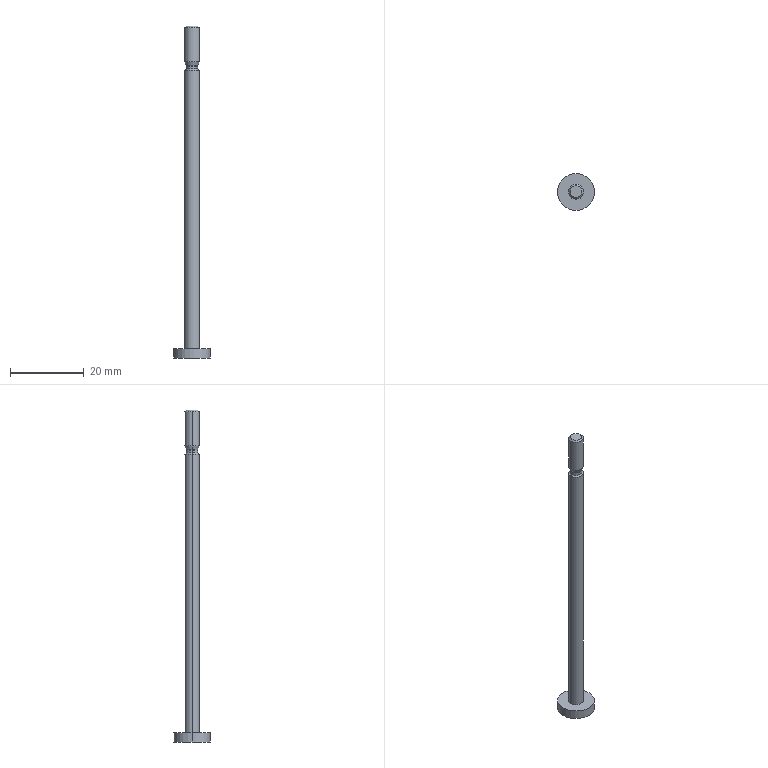Part | STEP file | PN_0050 | 1 solid | 19 faces | box 10 x 10 x 90 mm | volume 1287 mm3 | cylinder 8 | cone 4 | torus 4 | plane 3 | commonest cylinder face diameters 4 x4 3.2 x2 10 x2
STEP:
#1=CARTESIAN_POINT('',(0.,0.,0.));
#2=DIRECTION('',(0.,0.,1.));
#3=DIRECTION('',(1.,0.,0.));
#4=AXIS2_PLACEMENT_3D('',#1,#2,#3);
#5=CARTESIAN_POINT('',(1.571,0.,16.));
#6=VERTEX_POINT('',#5);
#7=CARTESIAN_POINT('',(-1.571,0.,16.));
#8=VERTEX_POINT('',#7);
#9=CARTESIAN_POINT('',(0.,0.,16.));
#10=DIRECTION('',(0.,0.,1.));
#11=DIRECTION('',(1.,0.,0.));
#12=AXIS2_PLACEMENT_3D('',#9,#10,#11);
#13=CIRCLE('',#12,1.571);
#14=CARTESIAN_POINT('',(0.,0.,15.57));
#15=DIRECTION('',(0.,0.,-1.));
#16=DIRECTION('',(-1.,0.,0.));
#17=AXIS2_PLACEMENT_3D('',#14,#15,#16);
#18=CONICAL_SURFACE('',#17,2.,0.7854);
#19=CARTESIAN_POINT('',(3.142,-0.4295));
#20=DIRECTION('',(-1.,0.));
#21=VECTOR('',#20,1.);
#22=LINE('',#19,#21);
#23=(GEOMETRIC_REPRESENTATION_CONTEXT(2)PARAMETRIC_REPRESENTATION_CONTEXT()REPRESENTATION_CONTEXT('',''));
#24=DEFINITIONAL_REPRESENTATION('',(#22),#23);
#25=PCURVE('',#18,#24);
#26=CARTESIAN_POINT('',(0.,0.,16.));
#27=DIRECTION('',(0.,0.,-1.));
#28=DIRECTION('',(-1.,0.,0.));
#29=AXIS2_PLACEMENT_3D('',#26,#27,#28);
#30=PLANE('',#29);
#31=CARTESIAN_POINT('',(-1.571,0.));
#32=CARTESIAN_POINT('',(-1.571,2.72));
#33=CARTESIAN_POINT('',(0.7853,1.36));
#34=CARTESIAN_POINT('',(3.141,0.));
#35=CARTESIAN_POINT('',(0.7853,-1.36));
#36=CARTESIAN_POINT('',(-1.571,-2.72));
#37=CARTESIAN_POINT('',(-1.571,0.));
#38=(BOUNDED_CURVE()B_SPLINE_CURVE(2,(#31,#32,#33,#34,#35,#36,#37),.UNSPECIFIED.,.T.,.F.)B_SPLINE_CURVE_WITH_KNOTS((1,2,2,2,2,1),(-2.094,0.,2.094,4.189,6.283,8.378),.UNSPECIFIED.)CURVE()GEOMETRIC_REPRESENTATION_ITEM()RATIONAL_B_SPLINE_CURVE((1.,0.5,1.,0.5,1.,0.5,1.))REPRESENTATION_ITEM(''));
#39=(GEOMETRIC_REPRESENTATION_CONTEXT(2)PARAMETRIC_REPRESENTATION_CONTEXT()REPRESENTATION_CONTEXT('',''));
#40=DEFINITIONAL_REPRESENTATION('',(#38),#39);
#41=PCURVE('',#30,#40);
#42=SURFACE_CURVE('',#13,(#25,#41),.PCURVE_S1.);
#43=EDGE_CURVE('',#6,#8,#42,.T.);
#44=ORIENTED_EDGE('',*,*,#43,.F.);
#45=CARTESIAN_POINT('',(2.,0.,15.57));
#46=VERTEX_POINT('',#45);
#47=CARTESIAN_POINT('',(2.,0.,15.57));
#48=DIRECTION('',(0.7071,0.,-0.7071));
#49=VECTOR('',#48,1.);
#50=LINE('',#47,#49);
#51=CARTESIAN_POINT('',(3.142,0.));
#52=DIRECTION('',(0.,1.));
#53=VECTOR('',#52,1.);
#54=LINE('',#51,#53);
#55=(GEOMETRIC_REPRESENTATION_CONTEXT(2)PARAMETRIC_REPRESENTATION_CONTEXT()REPRESENTATION_CONTEXT('',''));
#56=DEFINITIONAL_REPRESENTATION('',(#54),#55);
#57=PCURVE('',#18,#56);
#58=CARTESIAN_POINT('',(0.,0.,15.57));
#59=DIRECTION('',(0.,0.,-1.));
#60=DIRECTION('',(-1.,0.,0.));
#61=AXIS2_PLACEMENT_3D('',#58,#59,#60);
#62=CONICAL_SURFACE('',#61,2.,0.7854);
#63=CARTESIAN_POINT('',(3.142,0.));
#64=DIRECTION('',(0.,1.));
#65=VECTOR('',#64,1.);
#66=LINE('',#63,#65);
#67=(GEOMETRIC_REPRESENTATION_CONTEXT(2)PARAMETRIC_REPRESENTATION_CONTEXT()REPRESENTATION_CONTEXT('',''));
#68=DEFINITIONAL_REPRESENTATION('',(#66),#67);
#69=PCURVE('',#62,#68);
#70=SURFACE_CURVE('',#50,(#57,#69),.PCURVE_S1.);
#71=EDGE_CURVE('',#6,#46,#70,.T.);
#72=ORIENTED_EDGE('',*,*,#71,.T.);
#73=CARTESIAN_POINT('',(-2.,0.,15.57));
#74=VERTEX_POINT('',#73);
#75=CARTESIAN_POINT('',(0.,0.,15.57));
#76=DIRECTION('',(0.,0.,1.));
#77=DIRECTION('',(1.,0.,0.));
#78=AXIS2_PLACEMENT_3D('',#75,#76,#77);
#79=CIRCLE('',#78,2.);
#80=CARTESIAN_POINT('',(3.142,0.));
#81=DIRECTION('',(-1.,0.));
#82=VECTOR('',#81,1.);
#83=LINE('',#80,#82);
#84=(GEOMETRIC_REPRESENTATION_CONTEXT(2)PARAMETRIC_REPRESENTATION_CONTEXT()REPRESENTATION_CONTEXT('',''));
#85=DEFINITIONAL_REPRESENTATION('',(#83),#84);
#86=PCURVE('',#18,#85);
#87=CARTESIAN_POINT('',(0.,0.,3.));
#88=DIRECTION('',(0.,0.,1.));
#89=DIRECTION('',(1.,0.,0.));
#90=AXIS2_PLACEMENT_3D('',#87,#88,#89);
#91=CYLINDRICAL_SURFACE('',#90,2.);
#92=CARTESIAN_POINT('',(0.,12.57));
#93=DIRECTION('',(1.,0.));
#94=VECTOR('',#93,1.);
#95=LINE('',#92,#94);
#96=(GEOMETRIC_REPRESENTATION_CONTEXT(2)PARAMETRIC_REPRESENTATION_CONTEXT()REPRESENTATION_CONTEXT('',''));
#97=DEFINITIONAL_REPRESENTATION('',(#95),#96);
#98=PCURVE('',#91,#97);
#99=SURFACE_CURVE('',#79,(#86,#98),.PCURVE_S1.);
#100=EDGE_CURVE('',#46,#74,#99,.T.);
#101=ORIENTED_EDGE('',*,*,#100,.T.);
#102=CARTESIAN_POINT('',(-2.,0.,15.57));
#103=DIRECTION('',(-0.7071,0.,-0.7071));
#104=VECTOR('',#103,1.);
#105=LINE('',#102,#104);
#106=CARTESIAN_POINT('',(0.,0.));
#107=DIRECTION('',(0.,1.));
#108=VECTOR('',#107,1.);
#109=LINE('',#106,#108);
#110=(GEOMETRIC_REPRESENTATION_CONTEXT(2)PARAMETRIC_REPRESENTATION_CONTEXT()REPRESENTATION_CONTEXT('',''));
#111=DEFINITIONAL_REPRESENTATION('',(#109),#110);
#112=PCURVE('',#18,#111);
#113=CARTESIAN_POINT('',(6.283,0.));
#114=DIRECTION('',(0.,1.));
#115=VECTOR('',#114,1.);
#116=LINE('',#113,#115);
#117=(GEOMETRIC_REPRESENTATION_CONTEXT(2)PARAMETRIC_REPRESENTATION_CONTEXT()REPRESENTATION_CONTEXT('',''));
#118=DEFINITIONAL_REPRESENTATION('',(#116),#117);
#119=PCURVE('',#62,#118);
#120=SURFACE_CURVE('',#105,(#112,#119),.PCURVE_S1.);
#121=EDGE_CURVE('',#8,#74,#120,.T.);
#122=ORIENTED_EDGE('',*,*,#121,.F.);
#123=EDGE_LOOP('',(#44,#72,#101,#122));
#124=FACE_BOUND('',#123,.T.);
#125=ADVANCED_FACE('',(#124),#18,.T.);
#126=CARTESIAN_POINT('',(2.,0.,6.299));
#127=VERTEX_POINT('',#126);
#128=CARTESIAN_POINT('',(-2.,0.,6.299));
#129=VERTEX_POINT('',#128);
#130=CARTESIAN_POINT('',(0.,0.,6.299));
#131=DIRECTION('',(0.,0.,1.));
#132=DIRECTION('',(1.,0.,0.));
#133=AXIS2_PLACEMENT_3D('',#130,#131,#132);
#134=CIRCLE('',#133,2.);
#135=CARTESIAN_POINT('',(0.,3.299));
#136=DIRECTION('',(1.,0.));
#137=VECTOR('',#136,1.);
#138=LINE('',#135,#137);
#139=(GEOMETRIC_REPRESENTATION_CONTEXT(2)PARAMETRIC_REPRESENTATION_CONTEXT()REPRESENTATION_CONTEXT('',''));
#140=DEFINITIONAL_REPRESENTATION('',(#138),#139);
#141=PCURVE('',#91,#140);
#142=CARTESIAN_POINT('',(0.,0.,5.266));
#143=DIRECTION('',(0.,0.,1.));
#144=DIRECTION('',(1.,0.,0.));
#145=AXIS2_PLACEMENT_3D('',#142,#143,#144);
#146=CONICAL_SURFACE('',#145,1.624,0.3491);
#147=CARTESIAN_POINT('',(0.,1.033));
#148=DIRECTION('',(1.,0.));
#149=VECTOR('',#148,1.);
#150=LINE('',#147,#149);
#151=(GEOMETRIC_REPRESENTATION_CONTEXT(2)PARAMETRIC_REPRESENTATION_CONTEXT()REPRESENTATION_CONTEXT('',''));
#152=DEFINITIONAL_REPRESENTATION('',(#150),#151);
#153=PCURVE('',#146,#152);
#154=SURFACE_CURVE('',#134,(#141,#153),.PCURVE_S1.);
#155=EDGE_CURVE('',#127,#129,#154,.T.);
#156=ORIENTED_EDGE('',*,*,#155,.T.);
#157=CARTESIAN_POINT('',(-2.,0.,3.));
#158=DIRECTION('',(0.,0.,1.));
#159=VECTOR('',#158,1.);
#160=LINE('',#157,#159);
#161=CARTESIAN_POINT('',(3.142,0.));
#162=DIRECTION('',(0.,1.));
#163=VECTOR('',#162,1.);
#164=LINE('',#161,#163);
#165=(GEOMETRIC_REPRESENTATION_CONTEXT(2)PARAMETRIC_REPRESENTATION_CONTEXT()REPRESENTATION_CONTEXT('',''));
#166=DEFINITIONAL_REPRESENTATION('',(#164),#165);
#167=PCURVE('',#91,#166);
#168=CARTESIAN_POINT('',(0.,0.,3.));
#169=DIRECTION('',(0.,0.,1.));
#170=DIRECTION('',(1.,0.,0.));
#171=AXIS2_PLACEMENT_3D('',#168,#169,#170);
#172=CYLINDRICAL_SURFACE('',#171,2.);
#173=CARTESIAN_POINT('',(3.142,0.));
#174=DIRECTION('',(0.,1.));
#175=VECTOR('',#174,1.);
#176=LINE('',#173,#175);
#177=(GEOMETRIC_REPRESENTATION_CONTEXT(2)PARAMETRIC_REPRESENTATION_CONTEXT()REPRESENTATION_CONTEXT('',''));
#178=DEFINITIONAL_REPRESENTATION('',(#176),#177);
#179=PCURVE('',#172,#178);
#180=SURFACE_CURVE('',#160,(#167,#179),.PCURVE_S1.);
#181=EDGE_CURVE('',#129,#74,#180,.T.);
#182=ORIENTED_EDGE('',*,*,#181,.T.);
#183=ORIENTED_EDGE('',*,*,#100,.F.);
#184=CARTESIAN_POINT('',(2.,0.,3.));
#185=DIRECTION('',(0.,0.,1.));
#186=VECTOR('',#185,1.);
#187=LINE('',#184,#186);
#188=CARTESIAN_POINT('',(0.,0.));
#189=DIRECTION('',(0.,1.));
#190=VECTOR('',#189,1.);
#191=LINE('',#188,#190);
#192=(GEOMETRIC_REPRESENTATION_CONTEXT(2)PARAMETRIC_REPRESENTATION_CONTEXT()REPRESENTATION_CONTEXT('',''));
#193=DEFINITIONAL_REPRESENTATION('',(#191),#192);
#194=PCURVE('',#91,#193);
#195=CARTESIAN_POINT('',(6.283,0.));
#196=DIRECTION('',(0.,1.));
#197=VECTOR('',#196,1.);
#198=LINE('',#195,#197);
#199=(GEOMETRIC_REPRESENTATION_CONTEXT(2)PARAMETRIC_REPRESENTATION_CONTEXT()REPRESENTATION_CONTEXT('',''));
#200=DEFINITIONAL_REPRESENTATION('',(#198),#199);
#201=PCURVE('',#172,#200);
#202=SURFACE_CURVE('',#187,(#194,#201),.PCURVE_S1.);
#203=EDGE_CURVE('',#127,#46,#202,.T.);
#204=ORIENTED_EDGE('',*,*,#203,.F.);
#205=EDGE_LOOP('',(#156,#182,#183,#204));
#206=FACE_BOUND('',#205,.T.);
#207=ADVANCED_FACE('',(#206),#91,.T.);
#208=CARTESIAN_POINT('',(1.624,0.,5.266));
#209=VERTEX_POINT('',#208);
#210=CARTESIAN_POINT('',(-1.624,0.,5.266));
#211=VERTEX_POINT('',#210);
#212=CARTESIAN_POINT('',(0.,0.,5.266));
#213=DIRECTION('',(0.,0.,1.));
#214=DIRECTION('',(1.,0.,0.));
#215=AXIS2_PLACEMENT_3D('',#212,#213,#214);
#216=CIRCLE('',#215,1.624);
#217=CARTESIAN_POINT('',(0.,0.));
#218=DIRECTION('',(1.,0.));
#219=VECTOR('',#218,1.);
#220=LINE('',#217,#219);
#221=(GEOMETRIC_REPRESENTATION_CONTEXT(2)PARAMETRIC_REPRESENTATION_CONTEXT()REPRESENTATION_CONTEXT('',''));
#222=DEFINITIONAL_REPRESENTATION('',(#220),#221);
#223=PCURVE('',#146,#222);
#224=CARTESIAN_POINT('',(0.,0.,5.129));
#225=DIRECTION('',(0.,0.,1.));
#226=DIRECTION('',(1.,0.,0.));
#227=AXIS2_PLACEMENT_3D('',#224,#225,#226);
#228=TOROIDAL_SURFACE('',#227,2.,0.4);
#229=CARTESIAN_POINT('',(0.,2.793));
#230=DIRECTION('',(1.,0.));
#231=VECTOR('',#230,1.);
#232=LINE('',#229,#231);
#233=(GEOMETRIC_REPRESENTATION_CONTEXT(2)PARAMETRIC_REPRESENTATION_CONTEXT()REPRESENTATION_CONTEXT('',''));
#234=DEFINITIONAL_REPRESENTATION('',(#232),#233);
#235=PCURVE('',#228,#234);
#236=SURFACE_CURVE('',#216,(#223,#235),.PCURVE_S1.);
#237=EDGE_CURVE('',#209,#211,#236,.T.);
#238=ORIENTED_EDGE('',*,*,#237,.T.);
#239=CARTESIAN_POINT('',(-1.624,0.,5.266));
#240=DIRECTION('',(-0.342,0.,0.9397));
#241=VECTOR('',#240,1.);
#242=LINE('',#239,#241);
#243=CARTESIAN_POINT('',(3.142,0.));
#244=DIRECTION('',(0.,1.));
#245=VECTOR('',#244,1.);
#246=LINE('',#243,#245);
#247=(GEOMETRIC_REPRESENTATION_CONTEXT(2)PARAMETRIC_REPRESENTATION_CONTEXT()REPRESENTATION_CONTEXT('',''));
#248=DEFINITIONAL_REPRESENTATION('',(#246),#247);
#249=PCURVE('',#146,#248);
#250=CARTESIAN_POINT('',(0.,0.,5.266));
#251=DIRECTION('',(0.,0.,1.));
#252=DIRECTION('',(1.,0.,0.));
#253=AXIS2_PLACEMENT_3D('',#250,#251,#252);
#254=CONICAL_SURFACE('',#253,1.624,0.3491);
#255=CARTESIAN_POINT('',(3.142,0.));
#256=DIRECTION('',(0.,1.));
#257=VECTOR('',#256,1.);
#258=LINE('',#255,#257);
#259=(GEOMETRIC_REPRESENTATION_CONTEXT(2)PARAMETRIC_REPRESENTATION_CONTEXT()REPRESENTATION_CONTEXT('',''));
#260=DEFINITIONAL_REPRESENTATION('',(#258),#259);
#261=PCURVE('',#254,#260);
#262=SURFACE_CURVE('',#242,(#249,#261),.PCURVE_S1.);
#263=EDGE_CURVE('',#211,#129,#262,.T.);
#264=ORIENTED_EDGE('',*,*,#263,.T.);
#265=ORIENTED_EDGE('',*,*,#155,.F.);
#266=CARTESIAN_POINT('',(1.624,0.,5.266));
#267=DIRECTION('',(0.342,0.,0.9397));
#268=VECTOR('',#267,1.);
#269=LINE('',#266,#268);
#270=CARTESIAN_POINT('',(0.,0.));
#271=DIRECTION('',(0.,1.));
#272=VECTOR('',#271,1.);
#273=LINE('',#270,#272);
#274=(GEOMETRIC_REPRESENTATION_CONTEXT(2)PARAMETRIC_REPRESENTATION_CONTEXT()REPRESENTATION_CONTEXT('',''));
#275=DEFINITIONAL_REPRESENTATION('',(#273),#274);
#276=PCURVE('',#146,#275);
#277=CARTESIAN_POINT('',(6.283,0.));
#278=DIRECTION('',(0.,1.));
#279=VECTOR('',#278,1.);
#280=LINE('',#277,#279);
#281=(GEOMETRIC_REPRESENTATION_CONTEXT(2)PARAMETRIC_REPRESENTATION_CONTEXT()REPRESENTATION_CONTEXT('',''));
#282=DEFINITIONAL_REPRESENTATION('',(#280),#281);
#283=PCURVE('',#254,#282);
#284=SURFACE_CURVE('',#269,(#276,#283),.PCURVE_S1.);
#285=EDGE_CURVE('',#209,#127,#284,.T.);
#286=ORIENTED_EDGE('',*,*,#285,.F.);
#287=EDGE_LOOP('',(#238,#264,#265,#286));
#288=FACE_BOUND('',#287,.T.);
#289=ADVANCED_FACE('',(#288),#146,.T.);
#290=CARTESIAN_POINT('',(1.6,0.,5.129));
#291=VERTEX_POINT('',#290);
#292=CARTESIAN_POINT('',(2.,0.,5.129));
#293=DIRECTION('',(0.,-1.,0.));
#294=DIRECTION('',(0.,0.,-1.));
#295=AXIS2_PLACEMENT_3D('',#292,#293,#294);
#296=CIRCLE('',#295,0.4);
#297=CARTESIAN_POINT('',(0.,0.,5.129));
#298=DIRECTION('',(0.,0.,1.));
#299=DIRECTION('',(1.,0.,0.));
#300=AXIS2_PLACEMENT_3D('',#297,#298,#299);
#301=TOROIDAL_SURFACE('',#300,2.,0.4);
#302=CARTESIAN_POINT('',(6.283,-1.571));
#303=DIRECTION('',(0.,1.));
#304=VECTOR('',#303,1.);
#305=LINE('',#302,#304);
#306=(GEOMETRIC_REPRESENTATION_CONTEXT(2)PARAMETRIC_REPRESENTATION_CONTEXT()REPRESENTATION_CONTEXT('',''));
#307=DEFINITIONAL_REPRESENTATION('',(#305),#306);
#308=PCURVE('',#301,#307);
#309=CARTESIAN_POINT('',(0.,-1.571));
#310=DIRECTION('',(0.,1.));
#311=VECTOR('',#310,1.);
#312=LINE('',#309,#311);
#313=(GEOMETRIC_REPRESENTATION_CONTEXT(2)PARAMETRIC_REPRESENTATION_CONTEXT()REPRESENTATION_CONTEXT('',''));
#314=DEFINITIONAL_REPRESENTATION('',(#312),#313);
#315=PCURVE('',#228,#314);
#316=SURFACE_CURVE('',#296,(#308,#315),.PCURVE_S1.);
#317=EDGE_CURVE('',#209,#291,#316,.T.);
#318=ORIENTED_EDGE('',*,*,#317,.T.);
#319=CARTESIAN_POINT('',(-1.6,0.,5.129));
#320=VERTEX_POINT('',#319);
#321=CARTESIAN_POINT('',(0.,0.,5.129));
#322=DIRECTION('',(0.,0.,1.));
#323=DIRECTION('',(1.,0.,0.));
#324=AXIS2_PLACEMENT_3D('',#321,#322,#323);
#325=CIRCLE('',#324,1.6);
#326=CARTESIAN_POINT('',(0.,3.142));
#327=DIRECTION('',(1.,0.));
#328=VECTOR('',#327,1.);
#329=LINE('',#326,#328);
#330=(GEOMETRIC_REPRESENTATION_CONTEXT(2)PARAMETRIC_REPRESENTATION_CONTEXT()REPRESENTATION_CONTEXT('',''));
#331=DEFINITIONAL_REPRESENTATION('',(#329),#330);
#332=PCURVE('',#301,#331);
#333=CARTESIAN_POINT('',(0.,0.,3.));
#334=DIRECTION('',(0.,0.,1.));
#335=DIRECTION('',(1.,0.,0.));
#336=AXIS2_PLACEMENT_3D('',#333,#334,#335);
#337=CYLINDRICAL_SURFACE('',#336,1.6);
#338=CARTESIAN_POINT('',(0.,2.129));
#339=DIRECTION('',(1.,0.));
#340=VECTOR('',#339,1.);
#341=LINE('',#338,#340);
#342=(GEOMETRIC_REPRESENTATION_CONTEXT(2)PARAMETRIC_REPRESENTATION_CONTEXT()REPRESENTATION_CONTEXT('',''));
#343=DEFINITIONAL_REPRESENTATION('',(#341),#342);
#344=PCURVE('',#337,#343);
#345=SURFACE_CURVE('',#325,(#332,#344),.PCURVE_S1.);
#346=EDGE_CURVE('',#320,#291,#345,.T.);
#347=ORIENTED_EDGE('',*,*,#346,.F.);
#348=CARTESIAN_POINT('',(-2.,0.,5.129));
#349=DIRECTION('',(0.,1.,0.));
#350=DIRECTION('',(-1.,0.,0.));
#351=AXIS2_PLACEMENT_3D('',#348,#349,#350);
#352=CIRCLE('',#351,0.4);
#353=CARTESIAN_POINT('',(3.142,0.));
#354=DIRECTION('',(0.,1.));
#355=VECTOR('',#354,1.);
#356=LINE('',#353,#355);
#357=(GEOMETRIC_REPRESENTATION_CONTEXT(2)PARAMETRIC_REPRESENTATION_CONTEXT()REPRESENTATION_CONTEXT('',''));
#358=DEFINITIONAL_REPRESENTATION('',(#356),#357);
#359=PCURVE('',#301,#358);
#360=CARTESIAN_POINT('',(3.142,0.));
#361=DIRECTION('',(0.,1.));
#362=VECTOR('',#361,1.);
#363=LINE('',#360,#362);
#364=(GEOMETRIC_REPRESENTATION_CONTEXT(2)PARAMETRIC_REPRESENTATION_CONTEXT()REPRESENTATION_CONTEXT('',''));
#365=DEFINITIONAL_REPRESENTATION('',(#363),#364);
#366=PCURVE('',#228,#365);
#367=SURFACE_CURVE('',#352,(#359,#366),.PCURVE_S1.);
#368=EDGE_CURVE('',#211,#320,#367,.T.);
#369=ORIENTED_EDGE('',*,*,#368,.F.);
#370=CARTESIAN_POINT('',(0.,0.,5.266));
#371=DIRECTION('',(0.,0.,1.));
#372=DIRECTION('',(1.,0.,0.));
#373=AXIS2_PLACEMENT_3D('',#370,#371,#372);
#374=CIRCLE('',#373,1.624);
#375=CARTESIAN_POINT('',(0.,2.793));
#376=DIRECTION('',(1.,0.));
#377=VECTOR('',#376,1.);
#378=LINE('',#375,#377);
#379=(GEOMETRIC_REPRESENTATION_CONTEXT(2)PARAMETRIC_REPRESENTATION_CONTEXT()REPRESENTATION_CONTEXT('',''));
#380=DEFINITIONAL_REPRESENTATION('',(#378),#379);
#381=PCURVE('',#301,#380);
#382=CARTESIAN_POINT('',(0.,0.));
#383=DIRECTION('',(1.,0.));
#384=VECTOR('',#383,1.);
#385=LINE('',#382,#384);
#386=(GEOMETRIC_REPRESENTATION_CONTEXT(2)PARAMETRIC_REPRESENTATION_CONTEXT()REPRESENTATION_CONTEXT('',''));
#387=DEFINITIONAL_REPRESENTATION('',(#385),#386);
#388=PCURVE('',#254,#387);
#389=SURFACE_CURVE('',#374,(#381,#388),.PCURVE_S1.);
#390=EDGE_CURVE('',#211,#209,#389,.T.);
#391=ORIENTED_EDGE('',*,*,#390,.T.);
#392=EDGE_LOOP('',(#318,#347,#369,#391));
#393=FACE_BOUND('',#392,.F.);
#394=ADVANCED_FACE('',(#393),#301,.F.);
#395=CARTESIAN_POINT('',(1.6,0.,4.4));
#396=VERTEX_POINT('',#395);
#397=CARTESIAN_POINT('',(-1.6,0.,4.4));
#398=VERTEX_POINT('',#397);
#399=CARTESIAN_POINT('',(0.,0.,4.4));
#400=DIRECTION('',(0.,0.,1.));
#401=DIRECTION('',(1.,0.,0.));
#402=AXIS2_PLACEMENT_3D('',#399,#400,#401);
#403=CIRCLE('',#402,1.6);
#404=CARTESIAN_POINT('',(0.,0.,3.));
#405=DIRECTION('',(0.,0.,1.));
#406=DIRECTION('',(1.,0.,0.));
#407=AXIS2_PLACEMENT_3D('',#404,#405,#406);
#408=CYLINDRICAL_SURFACE('',#407,1.6);
#409=CARTESIAN_POINT('',(0.,1.4));
#410=DIRECTION('',(1.,0.));
#411=VECTOR('',#410,1.);
#412=LINE('',#409,#411);
#413=(GEOMETRIC_REPRESENTATION_CONTEXT(2)PARAMETRIC_REPRESENTATION_CONTEXT()REPRESENTATION_CONTEXT('',''));
#414=DEFINITIONAL_REPRESENTATION('',(#412),#413);
#415=PCURVE('',#408,#414);
#416=CARTESIAN_POINT('',(0.,0.,4.4));
#417=DIRECTION('',(0.,0.,1.));
#418=DIRECTION('',(1.,0.,0.));
#419=AXIS2_PLACEMENT_3D('',#416,#417,#418);
#420=TOROIDAL_SURFACE('',#419,2.,0.4);
#421=CARTESIAN_POINT('',(0.,3.142));
#422=DIRECTION('',(1.,0.));
#423=VECTOR('',#422,1.);
#424=LINE('',#421,#423);
#425=(GEOMETRIC_REPRESENTATION_CONTEXT(2)PARAMETRIC_REPRESENTATION_CONTEXT()REPRESENTATION_CONTEXT('',''));
#426=DEFINITIONAL_REPRESENTATION('',(#424),#425);
#427=PCURVE('',#420,#426);
#428=SURFACE_CURVE('',#403,(#415,#427),.PCURVE_S1.);
#429=EDGE_CURVE('',#396,#398,#428,.T.);
#430=ORIENTED_EDGE('',*,*,#429,.T.);
#431=CARTESIAN_POINT('',(-1.6,0.,3.));
#432=DIRECTION('',(0.,0.,1.));
#433=VECTOR('',#432,1.);
#434=LINE('',#431,#433);
#435=CARTESIAN_POINT('',(3.142,0.));
#436=DIRECTION('',(0.,1.));
#437=VECTOR('',#436,1.);
#438=LINE('',#435,#437);
#439=(GEOMETRIC_REPRESENTATION_CONTEXT(2)PARAMETRIC_REPRESENTATION_CONTEXT()REPRESENTATION_CONTEXT('',''));
#440=DEFINITIONAL_REPRESENTATION('',(#438),#439);
#441=PCURVE('',#408,#440);
#442=CARTESIAN_POINT('',(3.142,0.));
#443=DIRECTION('',(0.,1.));
#444=VECTOR('',#443,1.);
#445=LINE('',#442,#444);
#446=(GEOMETRIC_REPRESENTATION_CONTEXT(2)PARAMETRIC_REPRESENTATION_CONTEXT()REPRESENTATION_CONTEXT('',''));
#447=DEFINITIONAL_REPRESENTATION('',(#445),#446);
#448=PCURVE('',#337,#447);
#449=SURFACE_CURVE('',#434,(#441,#448),.PCURVE_S1.);
#450=EDGE_CURVE('',#398,#320,#449,.T.);
#451=ORIENTED_EDGE('',*,*,#450,.T.);
#452=CARTESIAN_POINT('',(0.,0.,5.129));
#453=DIRECTION('',(0.,0.,1.));
#454=DIRECTION('',(1.,0.,0.));
#455=AXIS2_PLACEMENT_3D('',#452,#453,#454);
#456=CIRCLE('',#455,1.6);
#457=CARTESIAN_POINT('',(0.,2.129));
#458=DIRECTION('',(1.,0.));
#459=VECTOR('',#458,1.);
#460=LINE('',#457,#459);
#461=(GEOMETRIC_REPRESENTATION_CONTEXT(2)PARAMETRIC_REPRESENTATION_CONTEXT()REPRESENTATION_CONTEXT('',''));
#462=DEFINITIONAL_REPRESENTATION('',(#460),#461);
#463=PCURVE('',#408,#462);
#464=CARTESIAN_POINT('',(0.,3.142));
#465=DIRECTION('',(1.,0.));
#466=VECTOR('',#465,1.);
#467=LINE('',#464,#466);
#468=(GEOMETRIC_REPRESENTATION_CONTEXT(2)PARAMETRIC_REPRESENTATION_CONTEXT()REPRESENTATION_CONTEXT('',''));
#469=DEFINITIONAL_REPRESENTATION('',(#467),#468);
#470=PCURVE('',#228,#469);
#471=SURFACE_CURVE('',#456,(#463,#470),.PCURVE_S1.);
#472=EDGE_CURVE('',#291,#320,#471,.T.);
#473=ORIENTED_EDGE('',*,*,#472,.F.);
#474=CARTESIAN_POINT('',(1.6,0.,3.));
#475=DIRECTION('',(0.,0.,1.));
#476=VECTOR('',#475,1.);
#477=LINE('',#474,#476);
#478=CARTESIAN_POINT('',(0.,0.));
#479=DIRECTION('',(0.,1.));
#480=VECTOR('',#479,1.);
#481=LINE('',#478,#480);
#482=(GEOMETRIC_REPRESENTATION_CONTEXT(2)PARAMETRIC_REPRESENTATION_CONTEXT()REPRESENTATION_CONTEXT('',''));
#483=DEFINITIONAL_REPRESENTATION('',(#481),#482);
#484=PCURVE('',#408,#483);
#485=CARTESIAN_POINT('',(6.283,0.));
#486=DIRECTION('',(0.,1.));
#487=VECTOR('',#486,1.);
#488=LINE('',#485,#487);
#489=(GEOMETRIC_REPRESENTATION_CONTEXT(2)PARAMETRIC_REPRESENTATION_CONTEXT()REPRESENTATION_CONTEXT('',''));
#490=DEFINITIONAL_REPRESENTATION('',(#488),#489);
#491=PCURVE('',#337,#490);
#492=SURFACE_CURVE('',#477,(#484,#491),.PCURVE_S1.);
#493=EDGE_CURVE('',#396,#291,#492,.T.);
#494=ORIENTED_EDGE('',*,*,#493,.F.);
#495=EDGE_LOOP('',(#430,#451,#473,#494));
#496=FACE_BOUND('',#495,.T.);
#497=ADVANCED_FACE('',(#496),#408,.T.);
#498=CARTESIAN_POINT('',(2.,0.,4.));
#499=VERTEX_POINT('',#498);
#500=CARTESIAN_POINT('',(2.,0.,4.4));
#501=DIRECTION('',(0.,-1.,0.));
#502=DIRECTION('',(0.,0.,-1.));
#503=AXIS2_PLACEMENT_3D('',#500,#501,#502);
#504=CIRCLE('',#503,0.4);
#505=CARTESIAN_POINT('',(0.,0.,4.4));
#506=DIRECTION('',(0.,0.,1.));
#507=DIRECTION('',(1.,0.,0.));
#508=AXIS2_PLACEMENT_3D('',#505,#506,#507);
#509=TOROIDAL_SURFACE('',#508,2.,0.4);
#510=CARTESIAN_POINT('',(6.283,-1.571));
#511=DIRECTION('',(0.,1.));
#512=VECTOR('',#511,1.);
#513=LINE('',#510,#512);
#514=(GEOMETRIC_REPRESENTATION_CONTEXT(2)PARAMETRIC_REPRESENTATION_CONTEXT()REPRESENTATION_CONTEXT('',''));
#515=DEFINITIONAL_REPRESENTATION('',(#513),#514);
#516=PCURVE('',#509,#515);
#517=CARTESIAN_POINT('',(0.,-1.571));
#518=DIRECTION('',(0.,1.));
#519=VECTOR('',#518,1.);
#520=LINE('',#517,#519);
#521=(GEOMETRIC_REPRESENTATION_CONTEXT(2)PARAMETRIC_REPRESENTATION_CONTEXT()REPRESENTATION_CONTEXT('',''));
#522=DEFINITIONAL_REPRESENTATION('',(#520),#521);
#523=PCURVE('',#420,#522);
#524=SURFACE_CURVE('',#504,(#516,#523),.PCURVE_S1.);
#525=EDGE_CURVE('',#396,#499,#524,.T.);
#526=ORIENTED_EDGE('',*,*,#525,.T.);
#527=CARTESIAN_POINT('',(-2.,0.,4.));
#528=VERTEX_POINT('',#527);
#529=CARTESIAN_POINT('',(0.,0.,4.));
#530=DIRECTION('',(0.,0.,1.));
#531=DIRECTION('',(1.,0.,0.));
#532=AXIS2_PLACEMENT_3D('',#529,#530,#531);
#533=CIRCLE('',#532,2.);
#534=CARTESIAN_POINT('',(0.,4.712));
#535=DIRECTION('',(1.,0.));
#536=VECTOR('',#535,1.);
#537=LINE('',#534,#536);
#538=(GEOMETRIC_REPRESENTATION_CONTEXT(2)PARAMETRIC_REPRESENTATION_CONTEXT()REPRESENTATION_CONTEXT('',''));
#539=DEFINITIONAL_REPRESENTATION('',(#537),#538);
#540=PCURVE('',#509,#539);
#541=CARTESIAN_POINT('',(0.,0.,-74.));
#542=DIRECTION('',(0.,0.,1.));
#543=DIRECTION('',(1.,0.,0.));
#544=AXIS2_PLACEMENT_3D('',#541,#542,#543);
#545=CYLINDRICAL_SURFACE('',#544,2.);
#546=CARTESIAN_POINT('',(0.,78.));
#547=DIRECTION('',(1.,0.));
#548=VECTOR('',#547,1.);
#549=LINE('',#546,#548);
#550=(GEOMETRIC_REPRESENTATION_CONTEXT(2)PARAMETRIC_REPRESENTATION_CONTEXT()REPRESENTATION_CONTEXT('',''));
#551=DEFINITIONAL_REPRESENTATION('',(#549),#550);
#552=PCURVE('',#545,#551);
#553=SURFACE_CURVE('',#533,(#540,#552),.PCURVE_S1.);
#554=EDGE_CURVE('',#528,#499,#553,.T.);
#555=ORIENTED_EDGE('',*,*,#554,.F.);
#556=CARTESIAN_POINT('',(-2.,0.,4.4));
#557=DIRECTION('',(0.,1.,0.));
#558=DIRECTION('',(-1.,0.,0.));
#559=AXIS2_PLACEMENT_3D('',#556,#557,#558);
#560=CIRCLE('',#559,0.4);
#561=CARTESIAN_POINT('',(3.142,0.));
#562=DIRECTION('',(0.,1.));
#563=VECTOR('',#562,1.);
#564=LINE('',#561,#563);
#565=(GEOMETRIC_REPRESENTATION_CONTEXT(2)PARAMETRIC_REPRESENTATION_CONTEXT()REPRESENTATION_CONTEXT('',''));
#566=DEFINITIONAL_REPRESENTATION('',(#564),#565);
#567=PCURVE('',#509,#566);
#568=CARTESIAN_POINT('',(3.142,0.));
#569=DIRECTION('',(0.,1.));
#570=VECTOR('',#569,1.);
#571=LINE('',#568,#570);
#572=(GEOMETRIC_REPRESENTATION_CONTEXT(2)PARAMETRIC_REPRESENTATION_CONTEXT()REPRESENTATION_CONTEXT('',''));
#573=DEFINITIONAL_REPRESENTATION('',(#571),#572);
#574=PCURVE('',#420,#573);
#575=SURFACE_CURVE('',#560,(#567,#574),.PCURVE_S1.);
#576=EDGE_CURVE('',#398,#528,#575,.T.);
#577=ORIENTED_EDGE('',*,*,#576,.F.);
#578=CARTESIAN_POINT('',(0.,0.,4.4));
#579=DIRECTION('',(0.,0.,1.));
#580=DIRECTION('',(1.,0.,0.));
#581=AXIS2_PLACEMENT_3D('',#578,#579,#580);
#582=CIRCLE('',#581,1.6);
#583=CARTESIAN_POINT('',(0.,3.142));
#584=DIRECTION('',(1.,0.));
#585=VECTOR('',#584,1.);
#586=LINE('',#583,#585);
#587=(GEOMETRIC_REPRESENTATION_CONTEXT(2)PARAMETRIC_REPRESENTATION_CONTEXT()REPRESENTATION_CONTEXT('',''));
#588=DEFINITIONAL_REPRESENTATION('',(#586),#587);
#589=PCURVE('',#509,#588);
#590=CARTESIAN_POINT('',(0.,1.4));
#591=DIRECTION('',(1.,0.));
#592=VECTOR('',#591,1.);
#593=LINE('',#590,#592);
#594=(GEOMETRIC_REPRESENTATION_CONTEXT(2)PARAMETRIC_REPRESENTATION_CONTEXT()REPRESENTATION_CONTEXT('',''));
#595=DEFINITIONAL_REPRESENTATION('',(#593),#594);
#596=PCURVE('',#337,#595);
#597=SURFACE_CURVE('',#582,(#589,#596),.PCURVE_S1.);
#598=EDGE_CURVE('',#398,#396,#597,.T.);
#599=ORIENTED_EDGE('',*,*,#598,.T.);
#600=EDGE_LOOP('',(#526,#555,#577,#599));
#601=FACE_BOUND('',#600,.F.);
#602=ADVANCED_FACE('',(#601),#509,.F.);
#603=CARTESIAN_POINT('',(5.,0.,-74.));
#604=VERTEX_POINT('',#603);
#605=CARTESIAN_POINT('',(-5.,0.,-74.));
#606=VERTEX_POINT('',#605);
#607=CARTESIAN_POINT('',(0.,0.,-74.));
#608=DIRECTION('',(0.,0.,1.));
#609=DIRECTION('',(1.,0.,0.));
#610=AXIS2_PLACEMENT_3D('',#607,#608,#609);
#611=CIRCLE('',#610,5.);
#612=CARTESIAN_POINT('',(0.,0.,-74.));
#613=DIRECTION('',(0.,0.,1.));
#614=DIRECTION('',(1.,0.,0.));
#615=AXIS2_PLACEMENT_3D('',#612,#613,#614);
#616=CYLINDRICAL_SURFACE('',#615,5.);
#617=CARTESIAN_POINT('',(0.,0.));
#618=DIRECTION('',(1.,0.));
#619=VECTOR('',#618,1.);
#620=LINE('',#617,#619);
#621=(GEOMETRIC_REPRESENTATION_CONTEXT(2)PARAMETRIC_REPRESENTATION_CONTEXT()REPRESENTATION_CONTEXT('',''));
#622=DEFINITIONAL_REPRESENTATION('',(#620),#621);
#623=PCURVE('',#616,#622);
#624=CARTESIAN_POINT('',(0.,5.,-74.));
#625=DIRECTION('',(0.,0.,1.));
#626=DIRECTION('',(1.,0.,0.));
#627=AXIS2_PLACEMENT_3D('',#624,#625,#626);
#628=PLANE('',#627);
#629=CARTESIAN_POINT('',(0.,-5.));
#630=DIRECTION('',(1.,0.));
#631=AXIS2_PLACEMENT_2D('',#629,#630);
#632=CIRCLE('',#631,5.);
#633=(GEOMETRIC_REPRESENTATION_CONTEXT(2)PARAMETRIC_REPRESENTATION_CONTEXT()REPRESENTATION_CONTEXT('',''));
#634=DEFINITIONAL_REPRESENTATION('',(#632),#633);
#635=PCURVE('',#628,#634);
#636=SURFACE_CURVE('',#611,(#623,#635),.PCURVE_S1.);
#637=EDGE_CURVE('',#604,#606,#636,.T.);
#638=ORIENTED_EDGE('',*,*,#637,.T.);
#639=CARTESIAN_POINT('',(-5.,0.,-71.5));
#640=VERTEX_POINT('',#639);
#641=CARTESIAN_POINT('',(-5.,0.,-74.));
#642=DIRECTION('',(0.,0.,1.));
#643=VECTOR('',#642,1.);
#644=LINE('',#641,#643);
#645=CARTESIAN_POINT('',(3.142,0.));
#646=DIRECTION('',(0.,1.));
#647=VECTOR('',#646,1.);
#648=LINE('',#645,#647);
#649=(GEOMETRIC_REPRESENTATION_CONTEXT(2)PARAMETRIC_REPRESENTATION_CONTEXT()REPRESENTATION_CONTEXT('',''));
#650=DEFINITIONAL_REPRESENTATION('',(#648),#649);
#651=PCURVE('',#616,#650);
#652=CARTESIAN_POINT('',(0.,0.,-74.));
#653=DIRECTION('',(0.,0.,1.));
#654=DIRECTION('',(1.,0.,0.));
#655=AXIS2_PLACEMENT_3D('',#652,#653,#654);
#656=CYLINDRICAL_SURFACE('',#655,5.);
#657=CARTESIAN_POINT('',(3.142,0.));
#658=DIRECTION('',(0.,1.));
#659=VECTOR('',#658,1.);
#660=LINE('',#657,#659);
#661=(GEOMETRIC_REPRESENTATION_CONTEXT(2)PARAMETRIC_REPRESENTATION_CONTEXT()REPRESENTATION_CONTEXT('',''));
#662=DEFINITIONAL_REPRESENTATION('',(#660),#661);
#663=PCURVE('',#656,#662);
#664=SURFACE_CURVE('',#644,(#651,#663),.PCURVE_S1.);
#665=EDGE_CURVE('',#606,#640,#664,.T.);
#666=ORIENTED_EDGE('',*,*,#665,.T.);
#667=CARTESIAN_POINT('',(5.,0.,-71.5));
#668=VERTEX_POINT('',#667);
#669=CARTESIAN_POINT('',(0.,0.,-71.5));
#670=DIRECTION('',(0.,0.,1.));
#671=DIRECTION('',(1.,0.,0.));
#672=AXIS2_PLACEMENT_3D('',#669,#670,#671);
#673=CIRCLE('',#672,5.);
#674=CARTESIAN_POINT('',(0.,2.5));
#675=DIRECTION('',(1.,0.));
#676=VECTOR('',#675,1.);
#677=LINE('',#674,#676);
#678=(GEOMETRIC_REPRESENTATION_CONTEXT(2)PARAMETRIC_REPRESENTATION_CONTEXT()REPRESENTATION_CONTEXT('',''));
#679=DEFINITIONAL_REPRESENTATION('',(#677),#678);
#680=PCURVE('',#616,#679);
#681=CARTESIAN_POINT('',(0.,2.,-71.5));
#682=DIRECTION('',(0.,0.,-1.));
#683=DIRECTION('',(-1.,0.,0.));
#684=AXIS2_PLACEMENT_3D('',#681,#682,#683);
#685=PLANE('',#684);
#686=CARTESIAN_POINT('',(-5.,-2.));
#687=CARTESIAN_POINT('',(-5.,6.66));
#688=CARTESIAN_POINT('',(2.5,2.33));
#689=CARTESIAN_POINT('',(10.,-2.));
#690=CARTESIAN_POINT('',(2.5,-6.33));
#691=CARTESIAN_POINT('',(-5.,-10.66));
#692=CARTESIAN_POINT('',(-5.,-2.));
#693=(BOUNDED_CURVE()B_SPLINE_CURVE(2,(#686,#687,#688,#689,#690,#691,#692),.UNSPECIFIED.,.T.,.F.)B_SPLINE_CURVE_WITH_KNOTS((1,2,2,2,2,1),(-2.094,0.,2.094,4.189,6.283,8.378),.UNSPECIFIED.)CURVE()GEOMETRIC_REPRESENTATION_ITEM()RATIONAL_B_SPLINE_CURVE((1.,0.5,1.,0.5,1.,0.5,1.))REPRESENTATION_ITEM(''));
#694=(GEOMETRIC_REPRESENTATION_CONTEXT(2)PARAMETRIC_REPRESENTATION_CONTEXT()REPRESENTATION_CONTEXT('',''));
#695=DEFINITIONAL_REPRESENTATION('',(#693),#694);
#696=PCURVE('',#685,#695);
#697=SURFACE_CURVE('',#673,(#680,#696),.PCURVE_S1.);
#698=EDGE_CURVE('',#668,#640,#697,.T.);
#699=ORIENTED_EDGE('',*,*,#698,.F.);
#700=CARTESIAN_POINT('',(5.,0.,-74.));
#701=DIRECTION('',(0.,0.,1.));
#702=VECTOR('',#701,1.);
#703=LINE('',#700,#702);
#704=CARTESIAN_POINT('',(0.,0.));
#705=DIRECTION('',(0.,1.));
#706=VECTOR('',#705,1.);
#707=LINE('',#704,#706);
#708=(GEOMETRIC_REPRESENTATION_CONTEXT(2)PARAMETRIC_REPRESENTATION_CONTEXT()REPRESENTATION_CONTEXT('',''));
#709=DEFINITIONAL_REPRESENTATION('',(#707),#708);
#710=PCURVE('',#616,#709);
#711=CARTESIAN_POINT('',(6.283,0.));
#712=DIRECTION('',(0.,1.));
#713=VECTOR('',#712,1.);
#714=LINE('',#711,#713);
#715=(GEOMETRIC_REPRESENTATION_CONTEXT(2)PARAMETRIC_REPRESENTATION_CONTEXT()REPRESENTATION_CONTEXT('',''));
#716=DEFINITIONAL_REPRESENTATION('',(#714),#715);
#717=PCURVE('',#656,#716);
#718=SURFACE_CURVE('',#703,(#710,#717),.PCURVE_S1.);
#719=EDGE_CURVE('',#604,#668,#718,.T.);
#720=ORIENTED_EDGE('',*,*,#719,.F.);
#721=EDGE_LOOP('',(#638,#666,#699,#720));
#722=FACE_BOUND('',#721,.T.);
#723=ADVANCED_FACE('',(#722),#616,.T.);
#724=CARTESIAN_POINT('',(2.,0.,-71.5));
#725=VERTEX_POINT('',#724);
#726=CARTESIAN_POINT('',(-2.,0.,-71.5));
#727=VERTEX_POINT('',#726);
#728=CARTESIAN_POINT('',(0.,0.,-71.5));
#729=DIRECTION('',(0.,0.,1.));
#730=DIRECTION('',(1.,0.,0.));
#731=AXIS2_PLACEMENT_3D('',#728,#729,#730);
#732=CIRCLE('',#731,2.);
#733=CARTESIAN_POINT('',(0.,0.,-74.));
#734=DIRECTION('',(0.,0.,1.));
#735=DIRECTION('',(1.,0.,0.));
#736=AXIS2_PLACEMENT_3D('',#733,#734,#735);
#737=CYLINDRICAL_SURFACE('',#736,2.);
#738=CARTESIAN_POINT('',(0.,2.5));
#739=DIRECTION('',(1.,0.));
#740=VECTOR('',#739,1.);
#741=LINE('',#738,#740);
#742=(GEOMETRIC_REPRESENTATION_CONTEXT(2)PARAMETRIC_REPRESENTATION_CONTEXT()REPRESENTATION_CONTEXT('',''));
#743=DEFINITIONAL_REPRESENTATION('',(#741),#742);
#744=PCURVE('',#737,#743);
#745=CARTESIAN_POINT('',(-2.,-2.));
#746=CARTESIAN_POINT('',(-2.,1.464));
#747=CARTESIAN_POINT('',(1.,-0.2679));
#748=CARTESIAN_POINT('',(4.,-2.));
#749=CARTESIAN_POINT('',(1.,-3.732));
#750=CARTESIAN_POINT('',(-2.,-5.464));
#751=CARTESIAN_POINT('',(-2.,-2.));
#752=(BOUNDED_CURVE()B_SPLINE_CURVE(2,(#745,#746,#747,#748,#749,#750,#751),.UNSPECIFIED.,.T.,.F.)B_SPLINE_CURVE_WITH_KNOTS((1,2,2,2,2,1),(-2.094,0.,2.094,4.189,6.283,8.378),.UNSPECIFIED.)CURVE()GEOMETRIC_REPRESENTATION_ITEM()RATIONAL_B_SPLINE_CURVE((1.,0.5,1.,0.5,1.,0.5,1.))REPRESENTATION_ITEM(''));
#753=(GEOMETRIC_REPRESENTATION_CONTEXT(2)PARAMETRIC_REPRESENTATION_CONTEXT()REPRESENTATION_CONTEXT('',''));
#754=DEFINITIONAL_REPRESENTATION('',(#752),#753);
#755=PCURVE('',#685,#754);
#756=SURFACE_CURVE('',#732,(#744,#755),.PCURVE_S1.);
#757=EDGE_CURVE('',#725,#727,#756,.T.);
#758=ORIENTED_EDGE('',*,*,#757,.T.);
#759=CARTESIAN_POINT('',(-2.,0.,-74.));
#760=DIRECTION('',(0.,0.,1.));
#761=VECTOR('',#760,1.);
#762=LINE('',#759,#761);
#763=CARTESIAN_POINT('',(3.142,0.));
#764=DIRECTION('',(0.,1.));
#765=VECTOR('',#764,1.);
#766=LINE('',#763,#765);
#767=(GEOMETRIC_REPRESENTATION_CONTEXT(2)PARAMETRIC_REPRESENTATION_CONTEXT()REPRESENTATION_CONTEXT('',''));
#768=DEFINITIONAL_REPRESENTATION('',(#766),#767);
#769=PCURVE('',#737,#768);
#770=CARTESIAN_POINT('',(3.142,0.));
#771=DIRECTION('',(0.,1.));
#772=VECTOR('',#771,1.);
#773=LINE('',#770,#772);
#774=(GEOMETRIC_REPRESENTATION_CONTEXT(2)PARAMETRIC_REPRESENTATION_CONTEXT()REPRESENTATION_CONTEXT('',''));
#775=DEFINITIONAL_REPRESENTATION('',(#773),#774);
#776=PCURVE('',#545,#775);
#777=SURFACE_CURVE('',#762,(#769,#776),.PCURVE_S1.);
#778=EDGE_CURVE('',#727,#528,#777,.T.);
#779=ORIENTED_EDGE('',*,*,#778,.T.);
#780=CARTESIAN_POINT('',(0.,0.,4.));
#781=DIRECTION('',(0.,0.,1.));
#782=DIRECTION('',(1.,0.,0.));
#783=AXIS2_PLACEMENT_3D('',#780,#781,#782);
#784=CIRCLE('',#783,2.);
#785=CARTESIAN_POINT('',(0.,78.));
#786=DIRECTION('',(1.,0.));
#787=VECTOR('',#786,1.);
#788=LINE('',#785,#787);
#789=(GEOMETRIC_REPRESENTATION_CONTEXT(2)PARAMETRIC_REPRESENTATION_CONTEXT()REPRESENTATION_CONTEXT('',''));
#790=DEFINITIONAL_REPRESENTATION('',(#788),#789);
#791=PCURVE('',#737,#790);
#792=CARTESIAN_POINT('',(0.,4.712));
#793=DIRECTION('',(1.,0.));
#794=VECTOR('',#793,1.);
#795=LINE('',#792,#794);
#796=(GEOMETRIC_REPRESENTATION_CONTEXT(2)PARAMETRIC_REPRESENTATION_CONTEXT()REPRESENTATION_CONTEXT('',''));
#797=DEFINITIONAL_REPRESENTATION('',(#795),#796);
#798=PCURVE('',#420,#797);
#799=SURFACE_CURVE('',#784,(#791,#798),.PCURVE_S1.);
#800=EDGE_CURVE('',#499,#528,#799,.T.);
#801=ORIENTED_EDGE('',*,*,#800,.F.);
#802=CARTESIAN_POINT('',(2.,0.,-74.));
#803=DIRECTION('',(0.,0.,1.));
#804=VECTOR('',#803,1.);
#805=LINE('',#802,#804);
#806=CARTESIAN_POINT('',(0.,0.));
#807=DIRECTION('',(0.,1.));
#808=VECTOR('',#807,1.);
#809=LINE('',#806,#808);
#810=(GEOMETRIC_REPRESENTATION_CONTEXT(2)PARAMETRIC_REPRESENTATION_CONTEXT()REPRESENTATION_CONTEXT('',''));
#811=DEFINITIONAL_REPRESENTATION('',(#809),#810);
#812=PCURVE('',#737,#811);
#813=CARTESIAN_POINT('',(6.283,0.));
#814=DIRECTION('',(0.,1.));
#815=VECTOR('',#814,1.);
#816=LINE('',#813,#815);
#817=(GEOMETRIC_REPRESENTATION_CONTEXT(2)PARAMETRIC_REPRESENTATION_CONTEXT()REPRESENTATION_CONTEXT('',''));
#818=DEFINITIONAL_REPRESENTATION('',(#816),#817);
#819=PCURVE('',#545,#818);
#820=SURFACE_CURVE('',#805,(#812,#819),.PCURVE_S1.);
#821=EDGE_CURVE('',#725,#499,#820,.T.);
#822=ORIENTED_EDGE('',*,*,#821,.F.);
#823=EDGE_LOOP('',(#758,#779,#801,#822));
#824=FACE_BOUND('',#823,.T.);
#825=ADVANCED_FACE('',(#824),#737,.T.);
#826=ORIENTED_EDGE('',*,*,#778,.F.);
#827=CARTESIAN_POINT('',(0.,0.,-71.5));
#828=DIRECTION('',(0.,0.,1.));
#829=DIRECTION('',(1.,0.,0.));
#830=AXIS2_PLACEMENT_3D('',#827,#828,#829);
#831=CIRCLE('',#830,2.);
#832=CARTESIAN_POINT('',(0.,2.5));
#833=DIRECTION('',(1.,0.));
#834=VECTOR('',#833,1.);
#835=LINE('',#832,#834);
#836=(GEOMETRIC_REPRESENTATION_CONTEXT(2)PARAMETRIC_REPRESENTATION_CONTEXT()REPRESENTATION_CONTEXT('',''));
#837=DEFINITIONAL_REPRESENTATION('',(#835),#836);
#838=PCURVE('',#545,#837);
#839=CARTESIAN_POINT('',(-2.,-2.));
#840=CARTESIAN_POINT('',(-2.,1.464));
#841=CARTESIAN_POINT('',(1.,-0.2679));
#842=CARTESIAN_POINT('',(4.,-2.));
#843=CARTESIAN_POINT('',(1.,-3.732));
#844=CARTESIAN_POINT('',(-2.,-5.464));
#845=CARTESIAN_POINT('',(-2.,-2.));
#846=(BOUNDED_CURVE()B_SPLINE_CURVE(2,(#839,#840,#841,#842,#843,#844,#845),.UNSPECIFIED.,.T.,.F.)B_SPLINE_CURVE_WITH_KNOTS((1,2,2,2,2,1),(-2.094,0.,2.094,4.189,6.283,8.378),.UNSPECIFIED.)CURVE()GEOMETRIC_REPRESENTATION_ITEM()RATIONAL_B_SPLINE_CURVE((1.,0.5,1.,0.5,1.,0.5,1.))REPRESENTATION_ITEM(''));
#847=(GEOMETRIC_REPRESENTATION_CONTEXT(2)PARAMETRIC_REPRESENTATION_CONTEXT()REPRESENTATION_CONTEXT('',''));
#848=DEFINITIONAL_REPRESENTATION('',(#846),#847);
#849=PCURVE('',#685,#848);
#850=SURFACE_CURVE('',#831,(#838,#849),.PCURVE_S1.);
#851=EDGE_CURVE('',#727,#725,#850,.T.);
#852=ORIENTED_EDGE('',*,*,#851,.T.);
#853=ORIENTED_EDGE('',*,*,#821,.T.);
#854=ORIENTED_EDGE('',*,*,#554,.F.);
#855=EDGE_LOOP('',(#826,#852,#853,#854));
#856=FACE_BOUND('',#855,.T.);
#857=ADVANCED_FACE('',(#856),#545,.T.);
#858=ORIENTED_EDGE('',*,*,#757,.F.);
#859=ORIENTED_EDGE('',*,*,#851,.F.);
#860=EDGE_LOOP('',(#858,#859));
#861=FACE_BOUND('',#860,.T.);
#862=ORIENTED_EDGE('',*,*,#698,.T.);
#863=CARTESIAN_POINT('',(0.,0.,-71.5));
#864=DIRECTION('',(0.,0.,1.));
#865=DIRECTION('',(1.,0.,0.));
#866=AXIS2_PLACEMENT_3D('',#863,#864,#865);
#867=CIRCLE('',#866,5.);
#868=CARTESIAN_POINT('',(-5.,-2.));
#869=CARTESIAN_POINT('',(-5.,6.66));
#870=CARTESIAN_POINT('',(2.5,2.33));
#871=CARTESIAN_POINT('',(10.,-2.));
#872=CARTESIAN_POINT('',(2.5,-6.33));
#873=CARTESIAN_POINT('',(-5.,-10.66));
#874=CARTESIAN_POINT('',(-5.,-2.));
#875=(BOUNDED_CURVE()B_SPLINE_CURVE(2,(#868,#869,#870,#871,#872,#873,#874),.UNSPECIFIED.,.T.,.F.)B_SPLINE_CURVE_WITH_KNOTS((1,2,2,2,2,1),(-2.094,0.,2.094,4.189,6.283,8.378),.UNSPECIFIED.)CURVE()GEOMETRIC_REPRESENTATION_ITEM()RATIONAL_B_SPLINE_CURVE((1.,0.5,1.,0.5,1.,0.5,1.))REPRESENTATION_ITEM(''));
#876=(GEOMETRIC_REPRESENTATION_CONTEXT(2)PARAMETRIC_REPRESENTATION_CONTEXT()REPRESENTATION_CONTEXT('',''));
#877=DEFINITIONAL_REPRESENTATION('',(#875),#876);
#878=PCURVE('',#685,#877);
#879=CARTESIAN_POINT('',(0.,2.5));
#880=DIRECTION('',(1.,0.));
#881=VECTOR('',#880,1.);
#882=LINE('',#879,#881);
#883=(GEOMETRIC_REPRESENTATION_CONTEXT(2)PARAMETRIC_REPRESENTATION_CONTEXT()REPRESENTATION_CONTEXT('',''));
#884=DEFINITIONAL_REPRESENTATION('',(#882),#883);
#885=PCURVE('',#656,#884);
#886=SURFACE_CURVE('',#867,(#878,#885),.PCURVE_S1.);
#887=EDGE_CURVE('',#640,#668,#886,.T.);
#888=ORIENTED_EDGE('',*,*,#887,.T.);
#889=EDGE_LOOP('',(#862,#888));
#890=FACE_BOUND('',#889,.T.);
#891=ADVANCED_FACE('',(#861,#890),#685,.F.);
#892=ORIENTED_EDGE('',*,*,#665,.F.);
#893=CARTESIAN_POINT('',(0.,0.,-74.));
#894=DIRECTION('',(0.,0.,1.));
#895=DIRECTION('',(1.,0.,0.));
#896=AXIS2_PLACEMENT_3D('',#893,#894,#895);
#897=CIRCLE('',#896,5.);
#898=CARTESIAN_POINT('',(0.,0.));
#899=DIRECTION('',(1.,0.));
#900=VECTOR('',#899,1.);
#901=LINE('',#898,#900);
#902=(GEOMETRIC_REPRESENTATION_CONTEXT(2)PARAMETRIC_REPRESENTATION_CONTEXT()REPRESENTATION_CONTEXT('',''));
#903=DEFINITIONAL_REPRESENTATION('',(#901),#902);
#904=PCURVE('',#656,#903);
#905=CARTESIAN_POINT('',(0.,-5.));
#906=DIRECTION('',(1.,0.));
#907=AXIS2_PLACEMENT_2D('',#905,#906);
#908=CIRCLE('',#907,5.);
#909=(GEOMETRIC_REPRESENTATION_CONTEXT(2)PARAMETRIC_REPRESENTATION_CONTEXT()REPRESENTATION_CONTEXT('',''));
#910=DEFINITIONAL_REPRESENTATION('',(#908),#909);
#911=PCURVE('',#628,#910);
#912=SURFACE_CURVE('',#897,(#904,#911),.PCURVE_S1.);
#913=EDGE_CURVE('',#606,#604,#912,.T.);
#914=ORIENTED_EDGE('',*,*,#913,.T.);
#915=ORIENTED_EDGE('',*,*,#719,.T.);
#916=ORIENTED_EDGE('',*,*,#887,.F.);
#917=EDGE_LOOP('',(#892,#914,#915,#916));
#918=FACE_BOUND('',#917,.T.);
#919=ADVANCED_FACE('',(#918),#656,.T.);
#920=ORIENTED_EDGE('',*,*,#637,.F.);
#921=ORIENTED_EDGE('',*,*,#913,.F.);
#922=EDGE_LOOP('',(#920,#921));
#923=FACE_BOUND('',#922,.T.);
#924=ADVANCED_FACE('',(#923),#628,.F.);
#925=ORIENTED_EDGE('',*,*,#800,.F.);
#926=ORIENTED_EDGE('',*,*,#525,.F.);
#927=ORIENTED_EDGE('',*,*,#429,.T.);
#928=ORIENTED_EDGE('',*,*,#576,.T.);
#929=EDGE_LOOP('',(#925,#926,#927,#928));
#930=FACE_BOUND('',#929,.F.);
#931=ADVANCED_FACE('',(#930),#420,.F.);
#932=ORIENTED_EDGE('',*,*,#450,.F.);
#933=ORIENTED_EDGE('',*,*,#598,.T.);
#934=ORIENTED_EDGE('',*,*,#493,.T.);
#935=ORIENTED_EDGE('',*,*,#346,.F.);
#936=EDGE_LOOP('',(#932,#933,#934,#935));
#937=FACE_BOUND('',#936,.T.);
#938=ADVANCED_FACE('',(#937),#337,.T.);
#939=ORIENTED_EDGE('',*,*,#472,.F.);
#940=ORIENTED_EDGE('',*,*,#317,.F.);
#941=ORIENTED_EDGE('',*,*,#237,.T.);
#942=ORIENTED_EDGE('',*,*,#368,.T.);
#943=EDGE_LOOP('',(#939,#940,#941,#942));
#944=FACE_BOUND('',#943,.F.);
#945=ADVANCED_FACE('',(#944),#228,.F.);
#946=ORIENTED_EDGE('',*,*,#263,.F.);
#947=ORIENTED_EDGE('',*,*,#390,.T.);
#948=ORIENTED_EDGE('',*,*,#285,.T.);
#949=CARTESIAN_POINT('',(0.,0.,6.299));
#950=DIRECTION('',(0.,0.,1.));
#951=DIRECTION('',(1.,0.,0.));
#952=AXIS2_PLACEMENT_3D('',#949,#950,#951);
#953=CIRCLE('',#952,2.);
#954=CARTESIAN_POINT('',(0.,1.033));
#955=DIRECTION('',(1.,0.));
#956=VECTOR('',#955,1.);
#957=LINE('',#954,#956);
#958=(GEOMETRIC_REPRESENTATION_CONTEXT(2)PARAMETRIC_REPRESENTATION_CONTEXT()REPRESENTATION_CONTEXT('',''));
#959=DEFINITIONAL_REPRESENTATION('',(#957),#958);
#960=PCURVE('',#254,#959);
#961=CARTESIAN_POINT('',(0.,3.299));
#962=DIRECTION('',(1.,0.));
#963=VECTOR('',#962,1.);
#964=LINE('',#961,#963);
#965=(GEOMETRIC_REPRESENTATION_CONTEXT(2)PARAMETRIC_REPRESENTATION_CONTEXT()REPRESENTATION_CONTEXT('',''));
#966=DEFINITIONAL_REPRESENTATION('',(#964),#965);
#967=PCURVE('',#172,#966);
#968=SURFACE_CURVE('',#953,(#960,#967),.PCURVE_S1.);
#969=EDGE_CURVE('',#129,#127,#968,.T.);
#970=ORIENTED_EDGE('',*,*,#969,.F.);
#971=EDGE_LOOP('',(#946,#947,#948,#970));
#972=FACE_BOUND('',#971,.T.);
#973=ADVANCED_FACE('',(#972),#254,.T.);
#974=ORIENTED_EDGE('',*,*,#181,.F.);
#975=ORIENTED_EDGE('',*,*,#969,.T.);
#976=ORIENTED_EDGE('',*,*,#203,.T.);
#977=CARTESIAN_POINT('',(0.,0.,15.57));
#978=DIRECTION('',(0.,0.,1.));
#979=DIRECTION('',(1.,0.,0.));
#980=AXIS2_PLACEMENT_3D('',#977,#978,#979);
#981=CIRCLE('',#980,2.);
#982=CARTESIAN_POINT('',(0.,12.57));
#983=DIRECTION('',(1.,0.));
#984=VECTOR('',#983,1.);
#985=LINE('',#982,#984);
#986=(GEOMETRIC_REPRESENTATION_CONTEXT(2)PARAMETRIC_REPRESENTATION_CONTEXT()REPRESENTATION_CONTEXT('',''));
#987=DEFINITIONAL_REPRESENTATION('',(#985),#986);
#988=PCURVE('',#172,#987);
#989=CARTESIAN_POINT('',(9.425,0.));
#990=DIRECTION('',(-1.,0.));
#991=VECTOR('',#990,1.);
#992=LINE('',#989,#991);
#993=(GEOMETRIC_REPRESENTATION_CONTEXT(2)PARAMETRIC_REPRESENTATION_CONTEXT()REPRESENTATION_CONTEXT('',''));
#994=DEFINITIONAL_REPRESENTATION('',(#992),#993);
#995=PCURVE('',#62,#994);
#996=SURFACE_CURVE('',#981,(#988,#995),.PCURVE_S1.);
#997=EDGE_CURVE('',#74,#46,#996,.T.);
#998=ORIENTED_EDGE('',*,*,#997,.F.);
#999=EDGE_LOOP('',(#974,#975,#976,#998));
#1000=FACE_BOUND('',#999,.T.);
#1001=ADVANCED_FACE('',(#1000),#172,.T.);
#1002=ORIENTED_EDGE('',*,*,#71,.F.);
#1003=CARTESIAN_POINT('',(0.,0.,16.));
#1004=DIRECTION('',(0.,0.,1.));
#1005=DIRECTION('',(1.,0.,0.));
#1006=AXIS2_PLACEMENT_3D('',#1003,#1004,#1005);
#1007=CIRCLE('',#1006,1.571);
#1008=CARTESIAN_POINT('',(9.425,-0.4295));
#1009=DIRECTION('',(-1.,0.));
#1010=VECTOR('',#1009,1.);
#1011=LINE('',#1008,#1010);
#1012=(GEOMETRIC_REPRESENTATION_CONTEXT(2)PARAMETRIC_REPRESENTATION_CONTEXT()REPRESENTATION_CONTEXT('',''));
#1013=DEFINITIONAL_REPRESENTATION('',(#1011),#1012);
#1014=PCURVE('',#62,#1013);
#1015=CARTESIAN_POINT('',(-1.571,0.));
#1016=CARTESIAN_POINT('',(-1.571,2.72));
#1017=CARTESIAN_POINT('',(0.7853,1.36));
#1018=CARTESIAN_POINT('',(3.141,0.));
#1019=CARTESIAN_POINT('',(0.7853,-1.36));
#1020=CARTESIAN_POINT('',(-1.571,-2.72));
#1021=CARTESIAN_POINT('',(-1.571,0.));
#1022=(BOUNDED_CURVE()B_SPLINE_CURVE(2,(#1015,#1016,#1017,#1018,#1019,#1020,#1021),.UNSPECIFIED.,.T.,.F.)B_SPLINE_CURVE_WITH_KNOTS((1,2,2,2,2,1),(-2.094,0.,2.094,4.189,6.283,8.378),.UNSPECIFIED.)CURVE()GEOMETRIC_REPRESENTATION_ITEM()RATIONAL_B_SPLINE_CURVE((1.,0.5,1.,0.5,1.,0.5,1.))REPRESENTATION_ITEM(''));
#1023=(GEOMETRIC_REPRESENTATION_CONTEXT(2)PARAMETRIC_REPRESENTATION_CONTEXT()REPRESENTATION_CONTEXT('',''));
#1024=DEFINITIONAL_REPRESENTATION('',(#1022),#1023);
#1025=PCURVE('',#30,#1024);
#1026=SURFACE_CURVE('',#1007,(#1014,#1025),.PCURVE_S1.);
#1027=EDGE_CURVE('',#8,#6,#1026,.T.);
#1028=ORIENTED_EDGE('',*,*,#1027,.F.);
#1029=ORIENTED_EDGE('',*,*,#121,.T.);
#1030=ORIENTED_EDGE('',*,*,#997,.T.);
#1031=EDGE_LOOP('',(#1002,#1028,#1029,#1030));
#1032=FACE_BOUND('',#1031,.T.);
#1033=ADVANCED_FACE('',(#1032),#62,.T.);
#1034=ORIENTED_EDGE('',*,*,#1027,.T.);
#1035=ORIENTED_EDGE('',*,*,#43,.T.);
#1036=EDGE_LOOP('',(#1034,#1035));
#1037=FACE_BOUND('',#1036,.T.);
#1038=ADVANCED_FACE('',(#1037),#30,.F.);
#1039=CLOSED_SHELL('',(#125,#207,#289,#394,#497,#602,#723,#825,#857,#891,#919,#924,#931,#938,#945,#973,#1001,#1033,#1038));
#1040=MANIFOLD_SOLID_BREP('',#1039);
#1041=(LENGTH_UNIT()NAMED_UNIT(*)SI_UNIT(.MILLI.,.METRE.));
#1042=UNCERTAINTY_MEASURE_WITH_UNIT(LENGTH_MEASURE(0.0000001),#1041,'','');
#1043=(NAMED_UNIT(*)PLANE_ANGLE_UNIT()SI_UNIT($,.RADIAN.));
#1044=(NAMED_UNIT(*)SI_UNIT($,.STERADIAN.)SOLID_ANGLE_UNIT());
#1045=(GEOMETRIC_REPRESENTATION_CONTEXT(3)GLOBAL_UNCERTAINTY_ASSIGNED_CONTEXT((#1042))GLOBAL_UNIT_ASSIGNED_CONTEXT((#1041,#1043,#1044))REPRESENTATION_CONTEXT('',''));
#1046=ADVANCED_BREP_SHAPE_REPRESENTATION('',(#4,#1040),#1045);